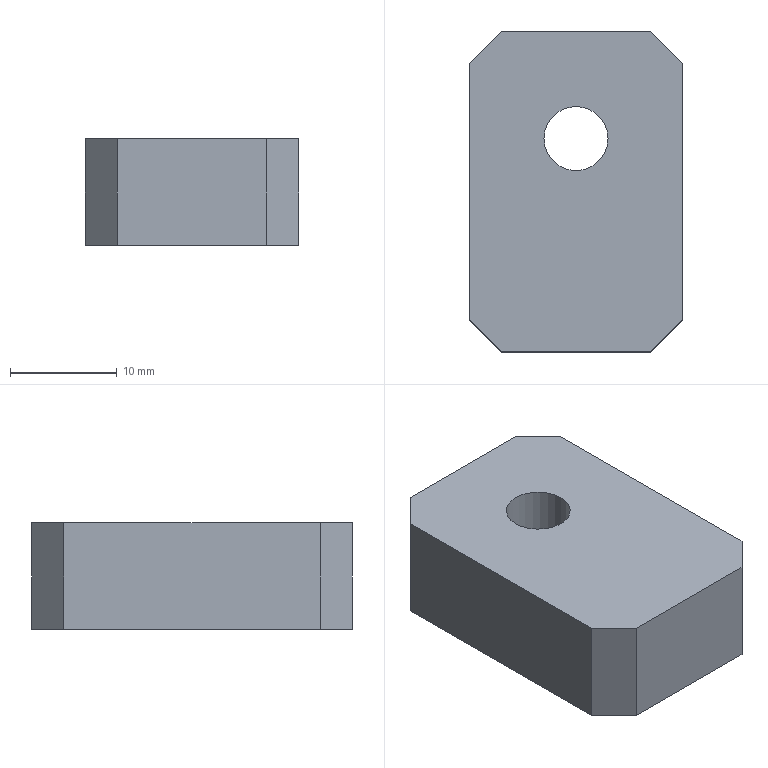Part | STEP file | solid 67 | 1 solid | 12 faces | box 20 x 30 x 10 mm | volume 5338 mm3 | plane 10 | cone 1 | cylinder 1 | commonest cylinder face diameters 6 x1